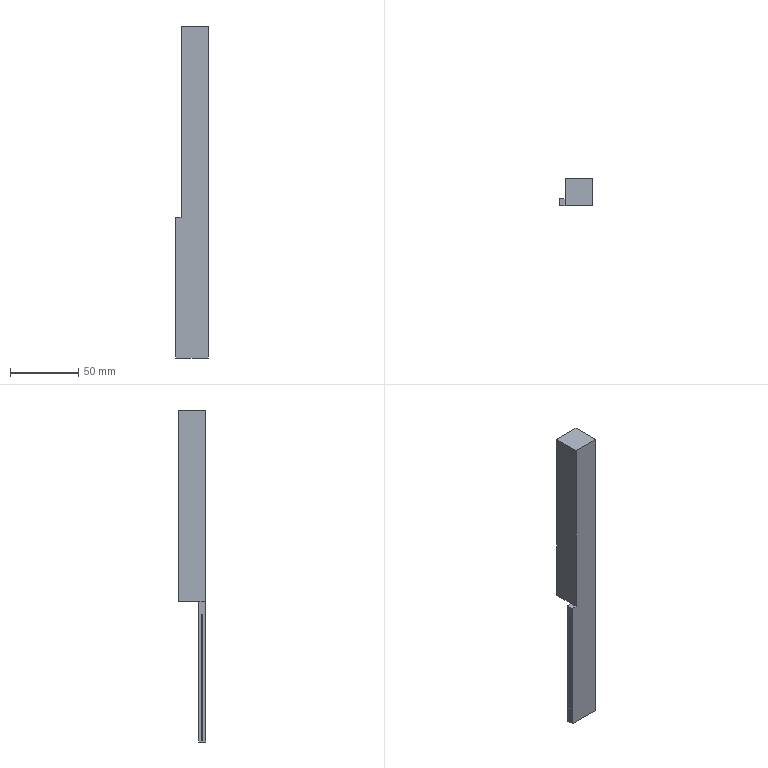Part | SolidWorks | features BaseBody 1 | 1 solid | 14 faces | box 24 x 20 x 243.345 mm | volume 68028 mm3 | plane 14
STEP:
#1=CARTESIAN_POINT('',(142.247,369.5,4.));
#2=VERTEX_POINT('',#1);
#3=CARTESIAN_POINT('',(122.247,369.5,4.));
#4=VERTEX_POINT('',#3);
#5=CARTESIAN_POINT('',(77.247,369.5,4.));
#6=DIRECTION('',(-1.,0.,0.));
#7=VECTOR('',#6,1000.);
#8=LINE('',#5,#7);
#9=EDGE_CURVE('',#2,#4,#8,.T.);
#10=ORIENTED_EDGE('',*,*,#9,.T.);
#11=CARTESIAN_POINT('',(122.247,369.5,-136.));
#12=VERTEX_POINT('',#11);
#13=CARTESIAN_POINT('',(122.247,369.5,-76.043));
#14=DIRECTION('',(0.,0.,-1.));
#15=VECTOR('',#14,1000.);
#16=LINE('',#13,#15);
#17=EDGE_CURVE('',#4,#12,#16,.T.);
#18=ORIENTED_EDGE('',*,*,#17,.T.);
#19=CARTESIAN_POINT('',(118.247,369.5,-136.));
#20=VERTEX_POINT('',#19);
#21=CARTESIAN_POINT('',(77.247,369.5,-136.));
#22=DIRECTION('',(-1.,0.,0.));
#23=VECTOR('',#22,1000.);
#24=LINE('',#21,#23);
#25=EDGE_CURVE('',#12,#20,#24,.T.);
#26=ORIENTED_EDGE('',*,*,#25,.T.);
#27=CARTESIAN_POINT('',(118.247,369.5,-239.345));
#28=VERTEX_POINT('',#27);
#29=CARTESIAN_POINT('',(118.247,369.5,-76.043));
#30=DIRECTION('',(0.,0.,-1.));
#31=VECTOR('',#30,1000.);
#32=LINE('',#29,#31);
#33=EDGE_CURVE('',#20,#28,#32,.T.);
#34=ORIENTED_EDGE('',*,*,#33,.T.);
#35=CARTESIAN_POINT('',(142.247,369.5,-239.345));
#36=VERTEX_POINT('',#35);
#37=CARTESIAN_POINT('',(77.247,369.5,-239.345));
#38=DIRECTION('',(1.,0.,0.));
#39=VECTOR('',#38,1000.);
#40=LINE('',#37,#39);
#41=EDGE_CURVE('',#28,#36,#40,.T.);
#42=ORIENTED_EDGE('',*,*,#41,.T.);
#43=CARTESIAN_POINT('',(142.247,369.5,-76.043));
#44=DIRECTION('',(0.,0.,1.));
#45=VECTOR('',#44,1000.);
#46=LINE('',#43,#45);
#47=EDGE_CURVE('',#36,#2,#46,.T.);
#48=ORIENTED_EDGE('',*,*,#47,.T.);
#49=EDGE_LOOP('',(#10,#18,#26,#34,#42,#48));
#50=FACE_OUTER_BOUND('',#49,.T.);
#51=CARTESIAN_POINT('',(77.247,369.5,-76.043));
#52=DIRECTION('',(0.,-1.,0.));
#53=DIRECTION('',(0.,0.,-1.));
#54=AXIS2_PLACEMENT_3D('',#51,#52,#53);
#55=PLANE('',#54);
#56=ADVANCED_FACE('',(#50),#55,.T.);
#57=ORIENTED_EDGE('',*,*,#17,.F.);
#58=CARTESIAN_POINT('',(122.247,389.5,4.));
#59=VERTEX_POINT('',#58);
#60=CARTESIAN_POINT('',(122.247,382.,4.));
#61=DIRECTION('',(0.,-1.,0.));
#62=VECTOR('',#61,1000.);
#63=LINE('',#60,#62);
#64=EDGE_CURVE('',#59,#4,#63,.T.);
#65=ORIENTED_EDGE('',*,*,#64,.F.);
#66=CARTESIAN_POINT('',(122.247,389.5,-136.));
#67=VERTEX_POINT('',#66);
#68=CARTESIAN_POINT('',(122.247,389.5,-76.043));
#69=DIRECTION('',(0.,0.,1.));
#70=VECTOR('',#69,1000.);
#71=LINE('',#68,#70);
#72=EDGE_CURVE('',#67,#59,#71,.T.);
#73=ORIENTED_EDGE('',*,*,#72,.F.);
#74=CARTESIAN_POINT('',(122.247,374.5,-136.));
#75=VERTEX_POINT('',#74);
#76=CARTESIAN_POINT('',(122.247,382.,-136.));
#77=DIRECTION('',(0.,1.,0.));
#78=VECTOR('',#77,1000.);
#79=LINE('',#76,#78);
#80=EDGE_CURVE('',#75,#67,#79,.T.);
#81=ORIENTED_EDGE('',*,*,#80,.F.);
#82=CARTESIAN_POINT('',(122.247,382.,-136.));
#83=DIRECTION('',(0.,1.,0.));
#84=VECTOR('',#83,1000.);
#85=LINE('',#82,#84);
#86=EDGE_CURVE('',#12,#75,#85,.T.);
#87=ORIENTED_EDGE('',*,*,#86,.F.);
#88=EDGE_LOOP('',(#57,#65,#73,#81,#87));
#89=FACE_OUTER_BOUND('',#88,.T.);
#90=CARTESIAN_POINT('',(122.247,382.,-76.043));
#91=DIRECTION('',(1.,0.,0.));
#92=DIRECTION('',(0.,0.,-1.));
#93=AXIS2_PLACEMENT_3D('',#90,#91,#92);
#94=PLANE('',#93);
#95=ADVANCED_FACE('',(#89),#94,.F.);
#96=CARTESIAN_POINT('',(142.247,389.5,4.));
#97=VERTEX_POINT('',#96);
#98=CARTESIAN_POINT('',(142.247,389.115,4.));
#99=DIRECTION('',(0.,1.,0.));
#100=VECTOR('',#99,1000.);
#101=LINE('',#98,#100);
#102=EDGE_CURVE('',#2,#97,#101,.T.);
#103=ORIENTED_EDGE('',*,*,#102,.T.);
#104=CARTESIAN_POINT('',(131.477,389.5,4.));
#105=DIRECTION('',(-1.,0.,0.));
#106=VECTOR('',#105,1000.);
#107=LINE('',#104,#106);
#108=EDGE_CURVE('',#97,#59,#107,.T.);
#109=ORIENTED_EDGE('',*,*,#108,.T.);
#110=ORIENTED_EDGE('',*,*,#64,.T.);
#111=ORIENTED_EDGE('',*,*,#9,.F.);
#112=EDGE_LOOP('',(#103,#109,#110,#111));
#113=FACE_OUTER_BOUND('',#112,.T.);
#114=CARTESIAN_POINT('',(131.477,389.115,4.));
#115=DIRECTION('',(0.,0.,1.));
#116=DIRECTION('',(1.,0.,0.));
#117=AXIS2_PLACEMENT_3D('',#114,#115,#116);
#118=PLANE('',#117);
#119=ADVANCED_FACE('',(#113),#118,.T.);
#120=ORIENTED_EDGE('',*,*,#102,.F.);
#121=ORIENTED_EDGE('',*,*,#47,.F.);
#122=CARTESIAN_POINT('',(142.247,374.5,-239.345));
#123=VERTEX_POINT('',#122);
#124=CARTESIAN_POINT('',(142.247,382.,-239.345));
#125=DIRECTION('',(0.,1.,0.));
#126=VECTOR('',#125,1000.);
#127=LINE('',#124,#126);
#128=EDGE_CURVE('',#36,#123,#127,.T.);
#129=ORIENTED_EDGE('',*,*,#128,.T.);
#130=CARTESIAN_POINT('',(142.247,374.5,-136.));
#131=VERTEX_POINT('',#130);
#132=CARTESIAN_POINT('',(142.247,374.5,-76.043));
#133=DIRECTION('',(0.,0.,1.));
#134=VECTOR('',#133,1000.);
#135=LINE('',#132,#134);
#136=EDGE_CURVE('',#123,#131,#135,.T.);
#137=ORIENTED_EDGE('',*,*,#136,.T.);
#138=CARTESIAN_POINT('',(142.247,389.5,-136.));
#139=VERTEX_POINT('',#138);
#140=CARTESIAN_POINT('',(142.247,382.,-136.));
#141=DIRECTION('',(0.,1.,0.));
#142=VECTOR('',#141,1000.);
#143=LINE('',#140,#142);
#144=EDGE_CURVE('',#131,#139,#143,.T.);
#145=ORIENTED_EDGE('',*,*,#144,.T.);
#146=CARTESIAN_POINT('',(142.247,389.5,-76.043));
#147=DIRECTION('',(0.,0.,1.));
#148=VECTOR('',#147,1000.);
#149=LINE('',#146,#148);
#150=EDGE_CURVE('',#139,#97,#149,.T.);
#151=ORIENTED_EDGE('',*,*,#150,.T.);
#152=EDGE_LOOP('',(#120,#121,#129,#137,#145,#151));
#153=FACE_OUTER_BOUND('',#152,.T.);
#154=CARTESIAN_POINT('',(142.247,382.,-76.043));
#155=DIRECTION('',(1.,0.,0.));
#156=DIRECTION('',(0.,0.,-1.));
#157=AXIS2_PLACEMENT_3D('',#154,#155,#156);
#158=PLANE('',#157);
#159=ADVANCED_FACE('',(#153),#158,.T.);
#160=CARTESIAN_POINT('',(118.247,371.5,-239.345));
#161=VERTEX_POINT('',#160);
#162=CARTESIAN_POINT('',(118.247,564.,-239.345));
#163=DIRECTION('',(0.,1.,0.));
#164=VECTOR('',#163,1000.);
#165=LINE('',#162,#164);
#166=EDGE_CURVE('',#28,#161,#165,.T.);
#167=ORIENTED_EDGE('',*,*,#166,.T.);
#168=CARTESIAN_POINT('',(122.247,371.5,-239.345));
#169=VERTEX_POINT('',#168);
#170=CARTESIAN_POINT('',(232.247,371.5,-239.345));
#171=DIRECTION('',(1.,0.,0.));
#172=VECTOR('',#171,1000.);
#173=LINE('',#170,#172);
#174=EDGE_CURVE('',#161,#169,#173,.T.);
#175=ORIENTED_EDGE('',*,*,#174,.T.);
#176=CARTESIAN_POINT('',(122.247,372.5,-239.345));
#177=VERTEX_POINT('',#176);
#178=CARTESIAN_POINT('',(122.247,564.,-239.345));
#179=DIRECTION('',(0.,1.,0.));
#180=VECTOR('',#179,1000.);
#181=LINE('',#178,#180);
#182=EDGE_CURVE('',#169,#177,#181,.T.);
#183=ORIENTED_EDGE('',*,*,#182,.T.);
#184=CARTESIAN_POINT('',(118.247,372.5,-239.345));
#185=VERTEX_POINT('',#184);
#186=CARTESIAN_POINT('',(232.247,372.5,-239.345));
#187=DIRECTION('',(-1.,0.,0.));
#188=VECTOR('',#187,1000.);
#189=LINE('',#186,#188);
#190=EDGE_CURVE('',#177,#185,#189,.T.);
#191=ORIENTED_EDGE('',*,*,#190,.T.);
#192=CARTESIAN_POINT('',(118.247,374.5,-239.345));
#193=VERTEX_POINT('',#192);
#194=CARTESIAN_POINT('',(118.247,564.,-239.345));
#195=DIRECTION('',(0.,1.,0.));
#196=VECTOR('',#195,1000.);
#197=LINE('',#194,#196);
#198=EDGE_CURVE('',#185,#193,#197,.T.);
#199=ORIENTED_EDGE('',*,*,#198,.T.);
#200=CARTESIAN_POINT('',(232.247,374.5,-239.345));
#201=DIRECTION('',(1.,0.,0.));
#202=VECTOR('',#201,1000.);
#203=LINE('',#200,#202);
#204=EDGE_CURVE('',#193,#123,#203,.T.);
#205=ORIENTED_EDGE('',*,*,#204,.T.);
#206=ORIENTED_EDGE('',*,*,#128,.F.);
#207=ORIENTED_EDGE('',*,*,#41,.F.);
#208=EDGE_LOOP('',(#167,#175,#183,#191,#199,#205,#206,#207));
#209=FACE_OUTER_BOUND('',#208,.T.);
#210=CARTESIAN_POINT('',(232.247,564.,-239.345));
#211=DIRECTION('',(0.,0.,-1.));
#212=DIRECTION('',(-1.,0.,0.));
#213=AXIS2_PLACEMENT_3D('',#210,#211,#212);
#214=PLANE('',#213);
#215=ADVANCED_FACE('',(#209),#214,.T.);
#216=ORIENTED_EDGE('',*,*,#166,.F.);
#217=ORIENTED_EDGE('',*,*,#33,.F.);
#218=CARTESIAN_POINT('',(118.247,374.5,-136.));
#219=VERTEX_POINT('',#218);
#220=CARTESIAN_POINT('',(118.247,382.,-136.));
#221=DIRECTION('',(0.,-1.,0.));
#222=VECTOR('',#221,1000.);
#223=LINE('',#220,#222);
#224=EDGE_CURVE('',#219,#20,#223,.T.);
#225=ORIENTED_EDGE('',*,*,#224,.F.);
#226=CARTESIAN_POINT('',(118.247,374.5,-76.043));
#227=DIRECTION('',(0.,0.,1.));
#228=VECTOR('',#227,1000.);
#229=LINE('',#226,#228);
#230=EDGE_CURVE('',#193,#219,#229,.T.);
#231=ORIENTED_EDGE('',*,*,#230,.F.);
#232=ORIENTED_EDGE('',*,*,#198,.F.);
#233=CARTESIAN_POINT('',(118.247,372.5,-146.043));
#234=VERTEX_POINT('',#233);
#235=CARTESIAN_POINT('',(118.247,372.5,-76.043));
#236=DIRECTION('',(0.,0.,-1.));
#237=VECTOR('',#236,1000.);
#238=LINE('',#235,#237);
#239=EDGE_CURVE('',#234,#185,#238,.T.);
#240=ORIENTED_EDGE('',*,*,#239,.F.);
#241=CARTESIAN_POINT('',(118.247,371.5,-146.043));
#242=VERTEX_POINT('',#241);
#243=CARTESIAN_POINT('',(118.247,382.,-146.043));
#244=DIRECTION('',(0.,1.,0.));
#245=VECTOR('',#244,1000.);
#246=LINE('',#243,#245);
#247=EDGE_CURVE('',#242,#234,#246,.T.);
#248=ORIENTED_EDGE('',*,*,#247,.F.);
#249=CARTESIAN_POINT('',(118.247,371.5,-76.043));
#250=DIRECTION('',(0.,0.,1.));
#251=VECTOR('',#250,1000.);
#252=LINE('',#249,#251);
#253=EDGE_CURVE('',#161,#242,#252,.T.);
#254=ORIENTED_EDGE('',*,*,#253,.F.);
#255=EDGE_LOOP('',(#216,#217,#225,#231,#232,#240,#248,#254));
#256=FACE_OUTER_BOUND('',#255,.T.);
#257=CARTESIAN_POINT('',(118.247,382.,-76.043));
#258=DIRECTION('',(1.,0.,0.));
#259=DIRECTION('',(0.,0.,-1.));
#260=AXIS2_PLACEMENT_3D('',#257,#258,#259);
#261=PLANE('',#260);
#262=ADVANCED_FACE('',(#256),#261,.F.);
#263=ORIENTED_EDGE('',*,*,#224,.T.);
#264=ORIENTED_EDGE('',*,*,#25,.F.);
#265=ORIENTED_EDGE('',*,*,#86,.T.);
#266=CARTESIAN_POINT('',(44.687,374.5,-136.));
#267=DIRECTION('',(1.,0.,0.));
#268=VECTOR('',#267,1000.);
#269=LINE('',#266,#268);
#270=EDGE_CURVE('',#219,#75,#269,.T.);
#271=ORIENTED_EDGE('',*,*,#270,.F.);
#272=EDGE_LOOP('',(#263,#264,#265,#271));
#273=FACE_OUTER_BOUND('',#272,.T.);
#274=CARTESIAN_POINT('',(44.687,379.5,-136.));
#275=DIRECTION('',(0.,0.,-1.));
#276=DIRECTION('',(-1.,0.,0.));
#277=AXIS2_PLACEMENT_3D('',#274,#275,#276);
#278=PLANE('',#277);
#279=ADVANCED_FACE('',(#273),#278,.F.);
#280=ORIENTED_EDGE('',*,*,#108,.F.);
#281=ORIENTED_EDGE('',*,*,#150,.F.);
#282=CARTESIAN_POINT('',(51.631,389.5,-136.));
#283=DIRECTION('',(-1.,0.,0.));
#284=VECTOR('',#283,1000.);
#285=LINE('',#282,#284);
#286=EDGE_CURVE('',#139,#67,#285,.T.);
#287=ORIENTED_EDGE('',*,*,#286,.T.);
#288=ORIENTED_EDGE('',*,*,#72,.T.);
#289=EDGE_LOOP('',(#280,#281,#287,#288));
#290=FACE_OUTER_BOUND('',#289,.T.);
#291=CARTESIAN_POINT('',(51.631,389.5,-344.615));
#292=DIRECTION('',(0.,1.,0.));
#293=DIRECTION('',(0.,0.,1.));
#294=AXIS2_PLACEMENT_3D('',#291,#292,#293);
#295=PLANE('',#294);
#296=ADVANCED_FACE('',(#290),#295,.T.);
#297=ORIENTED_EDGE('',*,*,#144,.F.);
#298=CARTESIAN_POINT('',(44.687,374.5,-136.));
#299=DIRECTION('',(-1.,0.,0.));
#300=VECTOR('',#299,1000.);
#301=LINE('',#298,#300);
#302=EDGE_CURVE('',#131,#75,#301,.T.);
#303=ORIENTED_EDGE('',*,*,#302,.T.);
#304=ORIENTED_EDGE('',*,*,#80,.T.);
#305=ORIENTED_EDGE('',*,*,#286,.F.);
#306=EDGE_LOOP('',(#297,#303,#304,#305));
#307=FACE_OUTER_BOUND('',#306,.T.);
#308=CARTESIAN_POINT('',(44.687,379.5,-136.));
#309=DIRECTION('',(0.,0.,-1.));
#310=DIRECTION('',(-1.,0.,0.));
#311=AXIS2_PLACEMENT_3D('',#308,#309,#310);
#312=PLANE('',#311);
#313=ADVANCED_FACE('',(#307),#312,.T.);
#314=ORIENTED_EDGE('',*,*,#136,.F.);
#315=ORIENTED_EDGE('',*,*,#204,.F.);
#316=ORIENTED_EDGE('',*,*,#230,.T.);
#317=ORIENTED_EDGE('',*,*,#270,.T.);
#318=ORIENTED_EDGE('',*,*,#302,.F.);
#319=EDGE_LOOP('',(#314,#315,#316,#317,#318));
#320=FACE_OUTER_BOUND('',#319,.T.);
#321=CARTESIAN_POINT('',(357.247,374.5,-344.345));
#322=DIRECTION('',(0.,-1.,0.));
#323=DIRECTION('',(0.,0.,-1.));
#324=AXIS2_PLACEMENT_3D('',#321,#322,#323);
#325=PLANE('',#324);
#326=ADVANCED_FACE('',(#320),#325,.F.);
#327=CARTESIAN_POINT('',(122.247,371.5,-146.043));
#328=VERTEX_POINT('',#327);
#329=CARTESIAN_POINT('',(57.247,371.5,-146.043));
#330=DIRECTION('',(-1.,0.,0.));
#331=VECTOR('',#330,1000.);
#332=LINE('',#329,#331);
#333=EDGE_CURVE('',#328,#242,#332,.T.);
#334=ORIENTED_EDGE('',*,*,#333,.F.);
#335=CARTESIAN_POINT('',(122.247,371.5,-276.043));
#336=DIRECTION('',(0.,0.,1.));
#337=VECTOR('',#336,1000.);
#338=LINE('',#335,#337);
#339=EDGE_CURVE('',#169,#328,#338,.T.);
#340=ORIENTED_EDGE('',*,*,#339,.F.);
#341=ORIENTED_EDGE('',*,*,#174,.F.);
#342=ORIENTED_EDGE('',*,*,#253,.T.);
#343=EDGE_LOOP('',(#334,#340,#341,#342));
#344=FACE_OUTER_BOUND('',#343,.T.);
#345=CARTESIAN_POINT('',(57.247,371.5,-276.043));
#346=DIRECTION('',(0.,-1.,0.));
#347=DIRECTION('',(0.,0.,-1.));
#348=AXIS2_PLACEMENT_3D('',#345,#346,#347);
#349=PLANE('',#348);
#350=ADVANCED_FACE('',(#344),#349,.F.);
#351=CARTESIAN_POINT('',(122.247,372.5,-146.043));
#352=VERTEX_POINT('',#351);
#353=CARTESIAN_POINT('',(57.247,372.5,-146.043));
#354=DIRECTION('',(1.,0.,0.));
#355=VECTOR('',#354,1000.);
#356=LINE('',#353,#355);
#357=EDGE_CURVE('',#234,#352,#356,.T.);
#358=ORIENTED_EDGE('',*,*,#357,.F.);
#359=ORIENTED_EDGE('',*,*,#239,.T.);
#360=ORIENTED_EDGE('',*,*,#190,.F.);
#361=CARTESIAN_POINT('',(122.247,372.5,-276.043));
#362=DIRECTION('',(0.,0.,-1.));
#363=VECTOR('',#362,1000.);
#364=LINE('',#361,#363);
#365=EDGE_CURVE('',#352,#177,#364,.T.);
#366=ORIENTED_EDGE('',*,*,#365,.F.);
#367=EDGE_LOOP('',(#358,#359,#360,#366));
#368=FACE_OUTER_BOUND('',#367,.T.);
#369=CARTESIAN_POINT('',(57.247,372.5,-276.043));
#370=DIRECTION('',(0.,1.,0.));
#371=DIRECTION('',(0.,0.,1.));
#372=AXIS2_PLACEMENT_3D('',#369,#370,#371);
#373=PLANE('',#372);
#374=ADVANCED_FACE('',(#368),#373,.F.);
#375=CARTESIAN_POINT('',(122.247,372.,-146.043));
#376=DIRECTION('',(0.,-1.,0.));
#377=VECTOR('',#376,1000.);
#378=LINE('',#375,#377);
#379=EDGE_CURVE('',#352,#328,#378,.T.);
#380=ORIENTED_EDGE('',*,*,#379,.F.);
#381=ORIENTED_EDGE('',*,*,#365,.T.);
#382=ORIENTED_EDGE('',*,*,#182,.F.);
#383=ORIENTED_EDGE('',*,*,#339,.T.);
#384=EDGE_LOOP('',(#380,#381,#382,#383));
#385=FACE_OUTER_BOUND('',#384,.T.);
#386=CARTESIAN_POINT('',(122.247,372.,-276.043));
#387=DIRECTION('',(1.,0.,0.));
#388=DIRECTION('',(0.,0.,-1.));
#389=AXIS2_PLACEMENT_3D('',#386,#387,#388);
#390=PLANE('',#389);
#391=ADVANCED_FACE('',(#385),#390,.F.);
#392=ORIENTED_EDGE('',*,*,#333,.T.);
#393=ORIENTED_EDGE('',*,*,#247,.T.);
#394=ORIENTED_EDGE('',*,*,#357,.T.);
#395=ORIENTED_EDGE('',*,*,#379,.T.);
#396=EDGE_LOOP('',(#392,#393,#394,#395));
#397=FACE_OUTER_BOUND('',#396,.T.);
#398=CARTESIAN_POINT('',(57.247,372.,-146.043));
#399=DIRECTION('',(0.,0.,1.));
#400=DIRECTION('',(1.,0.,0.));
#401=AXIS2_PLACEMENT_3D('',#398,#399,#400);
#402=PLANE('',#401);
#403=ADVANCED_FACE('',(#397),#402,.F.);
#404=CLOSED_SHELL('',(#56,#95,#119,#159,#215,#262,#279,#296,#313,#326,#350,#374,#391,#403));
#405=MANIFOLD_SOLID_BREP('',#404);
#406=CARTESIAN_POINT('',(0.,0.,0.));
#407=DIRECTION('',(0.,0.,1.));
#408=DIRECTION('',(1.,0.,0.));
#409=AXIS2_PLACEMENT_3D('',#406,#407,#408);
#410=(LENGTH_UNIT()NAMED_UNIT(*)SI_UNIT(.MILLI.,.METRE.));
#411=UNCERTAINTY_MEASURE_WITH_UNIT(LENGTH_MEASURE(0.00001),#410,'','');
#412=(NAMED_UNIT(*)PLANE_ANGLE_UNIT()SI_UNIT($,.RADIAN.));
#413=(NAMED_UNIT(*)SI_UNIT($,.STERADIAN.)SOLID_ANGLE_UNIT());
#414=(GEOMETRIC_REPRESENTATION_CONTEXT(3)GLOBAL_UNCERTAINTY_ASSIGNED_CONTEXT((#411))GLOBAL_UNIT_ASSIGNED_CONTEXT((#410,#412,#413))REPRESENTATION_CONTEXT('',''));
#415=ADVANCED_BREP_SHAPE_REPRESENTATION('',(#405,#409),#414);